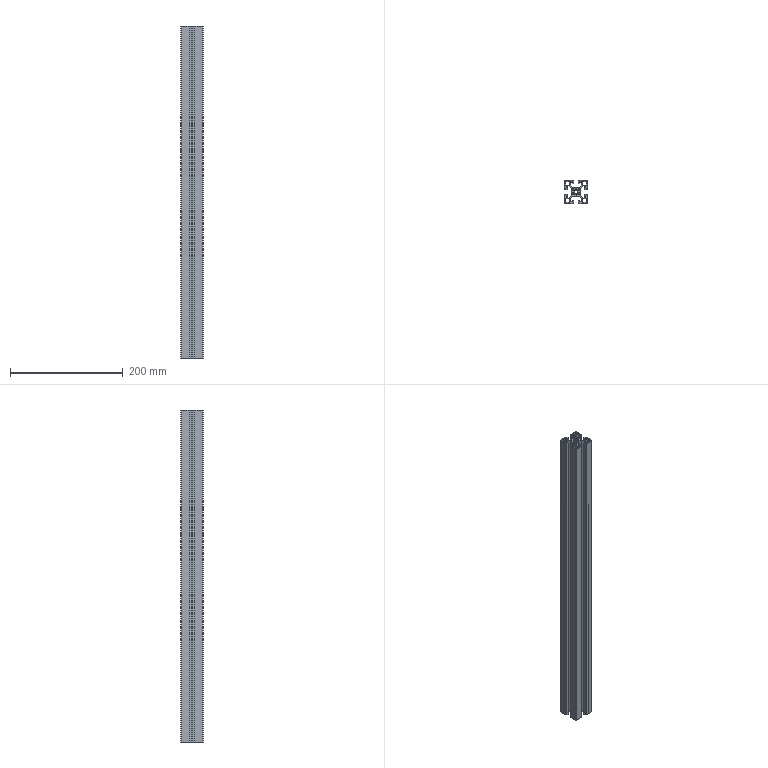Part | SolidWorks | features BaseBody 1, MoveFace 1 | 1 solid | 179 faces | box 40 x 40 x 588 mm | volume 315111 mm3 | plane 130 | cylinder 49 | commonest cylinder face diameters 0.6 x24 2 x8 10 x8 6.8 x5 3 x4